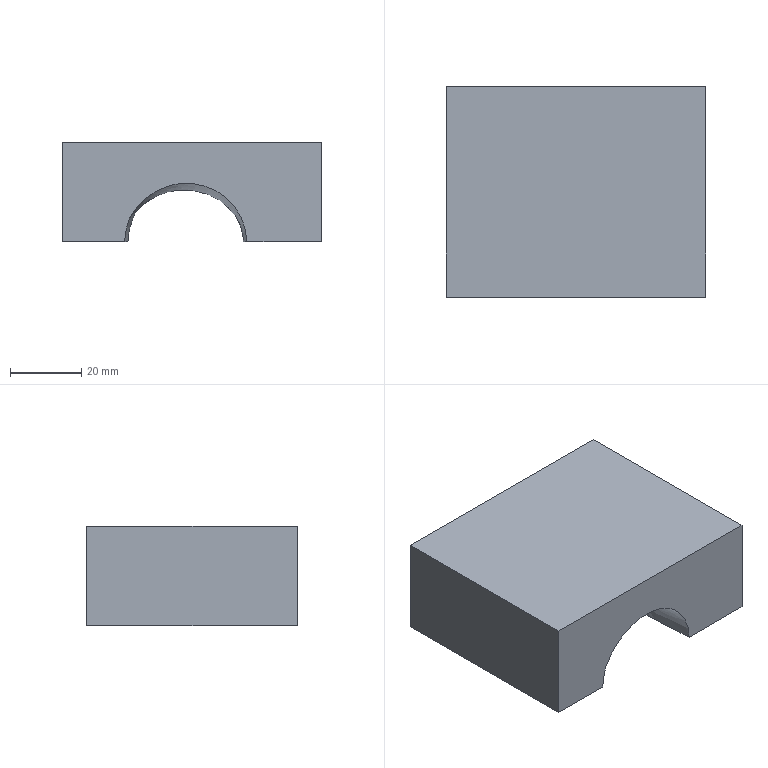NC program | NX | posted with a generic post | part box 72.744 x 59.015 x 27.972 mm
Lines 95882 to 95982 of 95982:
(ZLEVEL_PROFILE_1_COPY , TOOL : D6A45)
N191720 T01 M6
N191722 G54
N191724 G17 G0 G90 X-27.122 Y0. S9500 M3
N191726 G43 Z30. H1
N191728 Z1.5
N191730 G94 G1 Z-1. F1250.
N191732 G3 X-25.98 Y-1.141 R1.141
N191734 X-27.122 Y0. R-1.141
N191736 X-26.822 Y-0.52 R0.6
N191738 G1 Z0.5
N191740 G0 Z30.
N191742 X-26.786 Y-16.766
N191744 Z0.5
N191746 G1 Z-1.
N191748 X-27.722 Y-16.487
N191750 G3 X-28.022 Y-17.007 R0.6
N191752 X-25.98 Y-19.048 R2.041
N191754 X-28.022 Y-17.007 R-2.041
N191756 X-27.722 Y-17.527 R0.6
N191758 G1 X-26.786 Y-17.248
N191760 Z0.5
N191762 G0 Z30.
N191764 X23.842 Y1.319
N191766 Z1.5
N191768 G1 Z-1.
N191770 G3 X22.701 Y2.461 R1.141
N191772 X23.842 Y1.319 R-1.141
N191774 X23.542 Y1.839 R0.6
N191776 G1 Z0.5
N191778 G0 Z30.
N191780 X23.112 Y19.577
N191782 Z0.5
N191784 G1 Z-1.
N191786 X23.391 Y20.513
N191788 G3 X22.872 Y20.813 R0.6
N191790 X20.83 Y18.771 R2.041
N191792 X22.872 Y20.813 R-2.041
N191794 X22.352 Y20.513 R0.6
N191796 G1 X22.631 Y19.577
N191798 Z0.5
N191800 G0 Z30.
N191802 X38.53 Y1.035
N191804 Z0.5
N191806 G1 Z-1.
N191808 X37.63 Y0.516
N191810 G3 X37.33 Y-0.004 R0.6
N191812 G1 Y-29.518
N191814 G2 X36.374 Y-30.466 R0.952
N191816 G1 X15.544
N191818 G2 X14.625 Y-29.375 R0.933
N191820 G3 X15.283 Y-16. R55.516
N191822 X14.137 Y-3.357 R371.63
N191824 G2 X13.646 Y14.861 R113.246
N191826 G1 X14.436 Y29.575
N191828 G2 X15.376 Y30.466 R0.941
N191830 G1 X36.374
N191832 G2 X37.33 Y29.51 R0.979
N191834 G1 Y-0.004
N191836 G3 X37.63 Y-0.524 R0.6
N191838 G1 X38.53 Y-1.043
N191840 Z0.5
N191842 G0 Z30.
N191844 X-38.53
N191846 Z0.5
N191848 G1 Z-1.
N191850 X-37.63 Y-0.524
N191852 G3 X-37.33 Y-0.004 R0.6
N191854 G1 Y29.51
N191856 G2 X-36.374 Y30.466 R0.979
N191858 G1 X-18.854
N191860 G2 X-17.911 Y29.66 R0.97
N191862 X-17.167 Y22.898 R78.399
N191864 G1 X-17.164 Y22.9
N191866 X-17.137 Y22.493
N191868 Y22.412
N191870 G2 X-17.585 Y7.676 R79.929
N191872 G3 X-17.653 Y4.732 R16.814
N191874 G1 X-17.644 Y4.737
N191876 X-17.562 Y3.307
N191878 X-17.566 Y3.258
N191880 G2 X-19.437 Y-18.114 R79.751
N191882 G3 X-19.538 Y-19.062 R5.499
N191884 G1 X-19.283 Y-23.61
N191886 X-19.263 Y-23.939
N191888 X-19.254 Y-23.933
N191890 X-19.132 Y-25.13
N191892 X-19.137 Y-25.213
N191894 G3 X-18.499 Y-29.317 R66.02
N191896 G2 X-19.435 Y-30.466 R0.962
N191898 G1 X-36.374
N191900 G2 X-37.33 Y-29.518 R0.952
N191902 G1 Y-0.004
N191904 G3 X-37.63 Y0.516 R0.6
N191906 G1 X-38.53 Y1.035
N191908 Z0.5
N191910 G0 Z30.
N191912 M5
N191914 M2